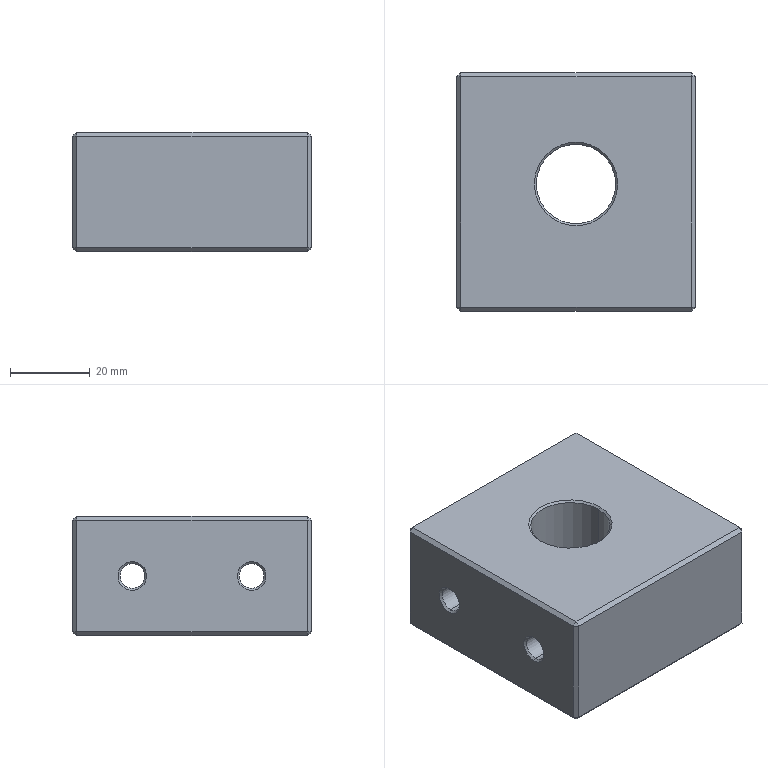Part | STEP file | 02-03 Driving mixing drum support seat | 1 solid | 59 faces | box 60 x 60 x 30 mm | volume 91539 mm3 | plane 29 | cone 18 | cylinder 12 | commonest cylinder face diameters 6.2 x4 10.5 x4 20 x2 24 x2